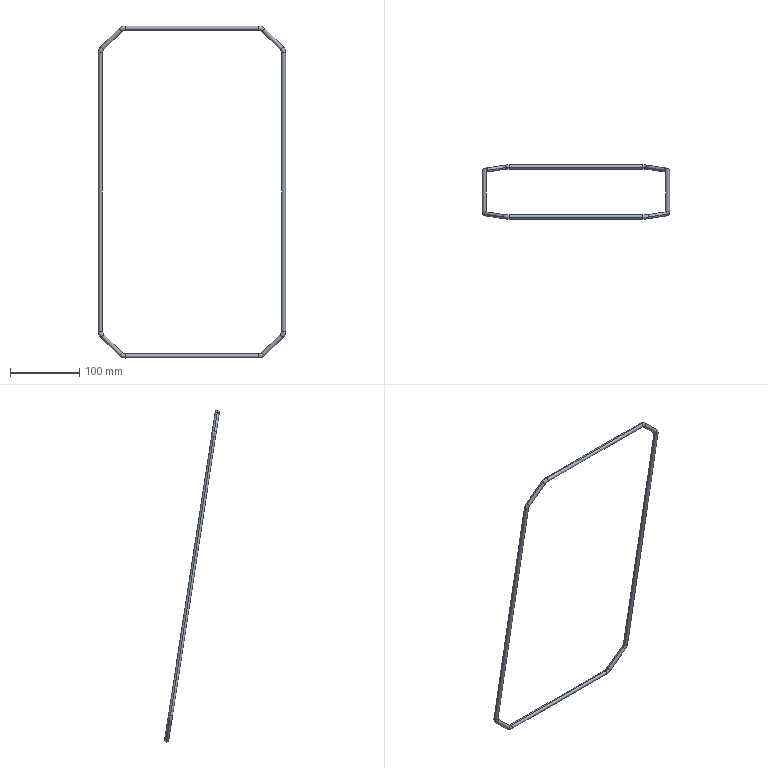Part | SolidWorks | features BaseBody 1 | 1 solid | 32 faces | box 271 x 79.199 x 480.386 mm | volume 39917 mm3 | torus 16 | cylinder 16 | commonest cylinder face diameters 6 x16
STEP:
#1=CARTESIAN_POINT('',(-509.93,505.658,-821.226));
#2=VERTEX_POINT('',#1);
#3=CARTESIAN_POINT('',(-513.445,504.364,-812.84));
#4=VERTEX_POINT('',#3);
#5=CARTESIAN_POINT('',(-501.445,504.364,-812.84));
#6=DIRECTION('',(0.,0.9883,0.1525));
#7=DIRECTION('',(-0.7071,0.1078,-0.6988));
#8=AXIS2_PLACEMENT_3D('',#5,#6,#7);
#9=CIRCLE('',#8,12.);
#10=EDGE_CURVE('',#2,#4,#9,.T.);
#11=ORIENTED_EDGE('',*,*,#10,.T.);
#12=CARTESIAN_POINT('',(-507.445,504.364,-812.84));
#13=VERTEX_POINT('',#12);
#14=CARTESIAN_POINT('',(-510.445,504.364,-812.84));
#15=DIRECTION('',(-0.000000028,-0.1525,0.9883));
#16=DIRECTION('',(1.,-0.000000004,0.000000028));
#17=AXIS2_PLACEMENT_3D('',#14,#15,#16);
#18=CIRCLE('',#17,3.);
#19=EDGE_CURVE('',#13,#4,#18,.T.);
#20=ORIENTED_EDGE('',*,*,#19,.F.);
#21=CARTESIAN_POINT('',(-505.688,505.011,-817.033));
#22=VERTEX_POINT('',#21);
#23=CARTESIAN_POINT('',(-501.445,504.364,-812.84));
#24=DIRECTION('',(0.,0.9883,0.1525));
#25=DIRECTION('',(-0.7071,0.1078,-0.6988));
#26=AXIS2_PLACEMENT_3D('',#23,#24,#25);
#27=CIRCLE('',#26,6.);
#28=EDGE_CURVE('',#22,#13,#27,.T.);
#29=ORIENTED_EDGE('',*,*,#28,.F.);
#30=CARTESIAN_POINT('',(-507.809,505.335,-819.13));
#31=DIRECTION('',(0.7071,0.1078,-0.6988));
#32=DIRECTION('',(-0.7071,0.1078,-0.6988));
#33=AXIS2_PLACEMENT_3D('',#30,#31,#32);
#34=CIRCLE('',#33,3.);
#35=EDGE_CURVE('',#2,#22,#34,.T.);
#36=ORIENTED_EDGE('',*,*,#35,.F.);
#37=EDGE_LOOP('',(#11,#20,#29,#36));
#38=FACE_OUTER_BOUND('',#37,.T.);
#39=CARTESIAN_POINT('',(-501.445,504.364,-812.84));
#40=DIRECTION('',(0.,0.9883,0.1525));
#41=DIRECTION('',(0.7071,-0.1078,0.6988));
#42=AXIS2_PLACEMENT_3D('',#39,#40,#41);
#43=TOROIDAL_SURFACE('',#42,9.,3.);
#44=ADVANCED_FACE('',(#38),#43,.T.);
#45=CARTESIAN_POINT('',(-483.134,509.744,-847.709));
#46=VERTEX_POINT('',#45);
#47=CARTESIAN_POINT('',(-483.134,509.744,-847.709));
#48=DIRECTION('',(-0.7071,-0.1078,0.6988));
#49=VECTOR('',#48,1000.);
#50=LINE('',#47,#49);
#51=EDGE_CURVE('',#46,#2,#50,.T.);
#52=ORIENTED_EDGE('',*,*,#51,.T.);
#53=ORIENTED_EDGE('',*,*,#35,.T.);
#54=CARTESIAN_POINT('',(-478.891,509.097,-843.516));
#55=VERTEX_POINT('',#54);
#56=CARTESIAN_POINT('',(-478.891,509.097,-843.516));
#57=DIRECTION('',(-0.7071,-0.1078,0.6988));
#58=VECTOR('',#57,1000.);
#59=LINE('',#56,#58);
#60=EDGE_CURVE('',#55,#22,#59,.T.);
#61=ORIENTED_EDGE('',*,*,#60,.F.);
#62=CARTESIAN_POINT('',(-481.013,509.421,-845.613));
#63=DIRECTION('',(-0.7071,-0.1078,0.6988));
#64=DIRECTION('',(0.7071,-0.1078,0.6988));
#65=AXIS2_PLACEMENT_3D('',#62,#63,#64);
#66=CIRCLE('',#65,3.);
#67=EDGE_CURVE('',#55,#46,#66,.T.);
#68=ORIENTED_EDGE('',*,*,#67,.T.);
#69=EDGE_LOOP('',(#52,#53,#61,#68));
#70=FACE_OUTER_BOUND('',#69,.T.);
#71=CARTESIAN_POINT('',(-481.013,509.421,-845.613));
#72=DIRECTION('',(-0.7071,-0.1078,0.6988));
#73=DIRECTION('',(-0.7071,0.1078,-0.6988));
#74=AXIS2_PLACEMENT_3D('',#71,#72,#73);
#75=CYLINDRICAL_SURFACE('',#74,3.);
#76=ADVANCED_FACE('',(#70),#75,.T.);
#77=CARTESIAN_POINT('',(-474.649,510.28,-851.183));
#78=VERTEX_POINT('',#77);
#79=CARTESIAN_POINT('',(-474.649,508.45,-839.323));
#80=DIRECTION('',(0.,0.9883,0.1525));
#81=DIRECTION('',(0.,0.1525,-0.9883));
#82=AXIS2_PLACEMENT_3D('',#79,#80,#81);
#83=CIRCLE('',#82,12.);
#84=EDGE_CURVE('',#78,#46,#83,.T.);
#85=ORIENTED_EDGE('',*,*,#84,.T.);
#86=ORIENTED_EDGE('',*,*,#67,.F.);
#87=CARTESIAN_POINT('',(-474.649,509.365,-845.253));
#88=VERTEX_POINT('',#87);
#89=CARTESIAN_POINT('',(-474.649,508.45,-839.323));
#90=DIRECTION('',(0.,0.9883,0.1525));
#91=DIRECTION('',(0.,0.1525,-0.9883));
#92=AXIS2_PLACEMENT_3D('',#89,#90,#91);
#93=CIRCLE('',#92,6.);
#94=EDGE_CURVE('',#88,#55,#93,.T.);
#95=ORIENTED_EDGE('',*,*,#94,.F.);
#96=CARTESIAN_POINT('',(-474.649,509.823,-848.218));
#97=DIRECTION('',(1.,0.,0.));
#98=DIRECTION('',(0.,0.1525,-0.9883));
#99=AXIS2_PLACEMENT_3D('',#96,#97,#98);
#100=CIRCLE('',#99,3.);
#101=EDGE_CURVE('',#78,#88,#100,.T.);
#102=ORIENTED_EDGE('',*,*,#101,.F.);
#103=EDGE_LOOP('',(#85,#86,#95,#102));
#104=FACE_OUTER_BOUND('',#103,.T.);
#105=CARTESIAN_POINT('',(-474.649,508.45,-839.323));
#106=DIRECTION('',(0.,0.9883,0.1525));
#107=DIRECTION('',(0.000000004,-0.1525,0.9883));
#108=AXIS2_PLACEMENT_3D('',#105,#106,#107);
#109=TOROIDAL_SURFACE('',#108,9.,3.);
#110=ADVANCED_FACE('',(#104),#109,.T.);
#111=CARTESIAN_POINT('',(-281.241,510.28,-851.183));
#112=VERTEX_POINT('',#111);
#113=CARTESIAN_POINT('',(-281.241,510.28,-851.183));
#114=DIRECTION('',(-1.,0.,0.));
#115=VECTOR('',#114,1000.);
#116=LINE('',#113,#115);
#117=EDGE_CURVE('',#112,#78,#116,.T.);
#118=ORIENTED_EDGE('',*,*,#117,.T.);
#119=ORIENTED_EDGE('',*,*,#101,.T.);
#120=CARTESIAN_POINT('',(-281.241,509.365,-845.253));
#121=VERTEX_POINT('',#120);
#122=CARTESIAN_POINT('',(-281.241,509.365,-845.253));
#123=DIRECTION('',(-1.,0.,0.));
#124=VECTOR('',#123,1000.);
#125=LINE('',#122,#124);
#126=EDGE_CURVE('',#121,#88,#125,.T.);
#127=ORIENTED_EDGE('',*,*,#126,.F.);
#128=CARTESIAN_POINT('',(-281.241,509.823,-848.218));
#129=DIRECTION('',(-1.,-0.000000001,0.000000004));
#130=DIRECTION('',(0.000000004,-0.1525,0.9883));
#131=AXIS2_PLACEMENT_3D('',#128,#129,#130);
#132=CIRCLE('',#131,3.);
#133=EDGE_CURVE('',#121,#112,#132,.T.);
#134=ORIENTED_EDGE('',*,*,#133,.T.);
#135=EDGE_LOOP('',(#118,#119,#127,#134));
#136=FACE_OUTER_BOUND('',#135,.T.);
#137=CARTESIAN_POINT('',(-281.241,509.823,-848.218));
#138=DIRECTION('',(-1.,0.,0.));
#139=DIRECTION('',(0.,0.1525,-0.9883));
#140=AXIS2_PLACEMENT_3D('',#137,#138,#139);
#141=CYLINDRICAL_SURFACE('',#140,3.);
#142=ADVANCED_FACE('',(#136),#141,.T.);
#143=CARTESIAN_POINT('',(-272.756,509.744,-847.709));
#144=VERTEX_POINT('',#143);
#145=CARTESIAN_POINT('',(-281.241,508.45,-839.323));
#146=DIRECTION('',(0.,0.9883,0.1525));
#147=DIRECTION('',(0.7071,0.1078,-0.6988));
#148=AXIS2_PLACEMENT_3D('',#145,#146,#147);
#149=CIRCLE('',#148,12.);
#150=EDGE_CURVE('',#144,#112,#149,.T.);
#151=ORIENTED_EDGE('',*,*,#150,.T.);
#152=ORIENTED_EDGE('',*,*,#133,.F.);
#153=CARTESIAN_POINT('',(-276.999,509.097,-843.516));
#154=VERTEX_POINT('',#153);
#155=CARTESIAN_POINT('',(-281.241,508.45,-839.323));
#156=DIRECTION('',(0.,0.9883,0.1525));
#157=DIRECTION('',(0.7071,0.1078,-0.6988));
#158=AXIS2_PLACEMENT_3D('',#155,#156,#157);
#159=CIRCLE('',#158,6.);
#160=EDGE_CURVE('',#154,#121,#159,.T.);
#161=ORIENTED_EDGE('',*,*,#160,.F.);
#162=CARTESIAN_POINT('',(-274.878,509.421,-845.613));
#163=DIRECTION('',(0.7071,-0.1078,0.6988));
#164=DIRECTION('',(0.7071,0.1078,-0.6988));
#165=AXIS2_PLACEMENT_3D('',#162,#163,#164);
#166=CIRCLE('',#165,3.);
#167=EDGE_CURVE('',#144,#154,#166,.T.);
#168=ORIENTED_EDGE('',*,*,#167,.F.);
#169=EDGE_LOOP('',(#151,#152,#161,#168));
#170=FACE_OUTER_BOUND('',#169,.T.);
#171=CARTESIAN_POINT('',(-281.241,508.45,-839.323));
#172=DIRECTION('',(0.,0.9883,0.1525));
#173=DIRECTION('',(-0.7071,-0.1078,0.6988));
#174=AXIS2_PLACEMENT_3D('',#171,#172,#173);
#175=TOROIDAL_SURFACE('',#174,9.,3.);
#176=ADVANCED_FACE('',(#170),#175,.T.);
#177=CARTESIAN_POINT('',(-245.96,505.658,-821.226));
#178=VERTEX_POINT('',#177);
#179=CARTESIAN_POINT('',(-245.96,505.658,-821.226));
#180=DIRECTION('',(-0.7071,0.1078,-0.6988));
#181=VECTOR('',#180,1000.);
#182=LINE('',#179,#181);
#183=EDGE_CURVE('',#178,#144,#182,.T.);
#184=ORIENTED_EDGE('',*,*,#183,.T.);
#185=ORIENTED_EDGE('',*,*,#167,.T.);
#186=CARTESIAN_POINT('',(-250.202,505.011,-817.033));
#187=VERTEX_POINT('',#186);
#188=CARTESIAN_POINT('',(-250.202,505.011,-817.033));
#189=DIRECTION('',(-0.7071,0.1078,-0.6988));
#190=VECTOR('',#189,1000.);
#191=LINE('',#188,#190);
#192=EDGE_CURVE('',#187,#154,#191,.T.);
#193=ORIENTED_EDGE('',*,*,#192,.F.);
#194=CARTESIAN_POINT('',(-248.081,505.335,-819.13));
#195=DIRECTION('',(-0.7071,0.1078,-0.6988));
#196=DIRECTION('',(-0.7071,-0.1078,0.6988));
#197=AXIS2_PLACEMENT_3D('',#194,#195,#196);
#198=CIRCLE('',#197,3.);
#199=EDGE_CURVE('',#187,#178,#198,.T.);
#200=ORIENTED_EDGE('',*,*,#199,.T.);
#201=EDGE_LOOP('',(#184,#185,#193,#200));
#202=FACE_OUTER_BOUND('',#201,.T.);
#203=CARTESIAN_POINT('',(-248.081,505.335,-819.13));
#204=DIRECTION('',(-0.7071,0.1078,-0.6988));
#205=DIRECTION('',(0.7071,0.1078,-0.6988));
#206=AXIS2_PLACEMENT_3D('',#203,#204,#205);
#207=CYLINDRICAL_SURFACE('',#206,3.);
#208=ADVANCED_FACE('',(#202),#207,.T.);
#209=CARTESIAN_POINT('',(-242.445,504.364,-812.84));
#210=VERTEX_POINT('',#209);
#211=CARTESIAN_POINT('',(-254.445,504.364,-812.84));
#212=DIRECTION('',(0.,0.9883,0.1525));
#213=DIRECTION('',(1.,0.,0.));
#214=AXIS2_PLACEMENT_3D('',#211,#212,#213);
#215=CIRCLE('',#214,12.);
#216=EDGE_CURVE('',#210,#178,#215,.T.);
#217=ORIENTED_EDGE('',*,*,#216,.T.);
#218=ORIENTED_EDGE('',*,*,#199,.F.);
#219=CARTESIAN_POINT('',(-248.445,504.364,-812.84));
#220=VERTEX_POINT('',#219);
#221=CARTESIAN_POINT('',(-254.445,504.364,-812.84));
#222=DIRECTION('',(0.,0.9883,0.1525));
#223=DIRECTION('',(1.,0.,0.));
#224=AXIS2_PLACEMENT_3D('',#221,#222,#223);
#225=CIRCLE('',#224,6.);
#226=EDGE_CURVE('',#220,#187,#225,.T.);
#227=ORIENTED_EDGE('',*,*,#226,.F.);
#228=CARTESIAN_POINT('',(-245.445,504.364,-812.84));
#229=DIRECTION('',(0.,-0.1525,0.9883));
#230=DIRECTION('',(1.,0.,0.));
#231=AXIS2_PLACEMENT_3D('',#228,#229,#230);
#232=CIRCLE('',#231,3.);
#233=EDGE_CURVE('',#210,#220,#232,.T.);
#234=ORIENTED_EDGE('',*,*,#233,.F.);
#235=EDGE_LOOP('',(#217,#218,#227,#234));
#236=FACE_OUTER_BOUND('',#235,.T.);
#237=CARTESIAN_POINT('',(-254.445,504.364,-812.84));
#238=DIRECTION('',(0.,0.9883,0.1525));
#239=DIRECTION('',(-1.,-0.000000002,0.000000011));
#240=AXIS2_PLACEMENT_3D('',#237,#238,#239);
#241=TOROIDAL_SURFACE('',#240,9.,3.);
#242=ADVANCED_FACE('',(#236),#241,.T.);
#243=CARTESIAN_POINT('',(-242.445,442.083,-409.21));
#244=VERTEX_POINT('',#243);
#245=CARTESIAN_POINT('',(-242.445,442.083,-409.21));
#246=DIRECTION('',(0.,0.1525,-0.9883));
#247=VECTOR('',#246,1000.);
#248=LINE('',#245,#247);
#249=EDGE_CURVE('',#244,#210,#248,.T.);
#250=ORIENTED_EDGE('',*,*,#249,.T.);
#251=ORIENTED_EDGE('',*,*,#233,.T.);
#252=CARTESIAN_POINT('',(-248.445,442.083,-409.21));
#253=VERTEX_POINT('',#252);
#254=CARTESIAN_POINT('',(-248.445,442.083,-409.21));
#255=DIRECTION('',(0.,0.1525,-0.9883));
#256=VECTOR('',#255,1000.);
#257=LINE('',#254,#256);
#258=EDGE_CURVE('',#253,#220,#257,.T.);
#259=ORIENTED_EDGE('',*,*,#258,.F.);
#260=CARTESIAN_POINT('',(-245.445,442.083,-409.21));
#261=DIRECTION('',(-0.000000004,0.1525,-0.9883));
#262=DIRECTION('',(-1.,-0.000000001,0.000000004));
#263=AXIS2_PLACEMENT_3D('',#260,#261,#262);
#264=CIRCLE('',#263,3.);
#265=EDGE_CURVE('',#253,#244,#264,.T.);
#266=ORIENTED_EDGE('',*,*,#265,.T.);
#267=EDGE_LOOP('',(#250,#251,#259,#266));
#268=FACE_OUTER_BOUND('',#267,.T.);
#269=CARTESIAN_POINT('',(-245.445,442.083,-409.21));
#270=DIRECTION('',(0.,0.1525,-0.9883));
#271=DIRECTION('',(1.,0.,0.));
#272=AXIS2_PLACEMENT_3D('',#269,#270,#271);
#273=CYLINDRICAL_SURFACE('',#272,3.);
#274=ADVANCED_FACE('',(#268),#273,.T.);
#275=CARTESIAN_POINT('',(-245.96,440.789,-400.823));
#276=VERTEX_POINT('',#275);
#277=CARTESIAN_POINT('',(-254.445,442.083,-409.21));
#278=DIRECTION('',(0.,0.9883,0.1525));
#279=DIRECTION('',(0.7071,-0.1078,0.6988));
#280=AXIS2_PLACEMENT_3D('',#277,#278,#279);
#281=CIRCLE('',#280,12.);
#282=EDGE_CURVE('',#276,#244,#281,.T.);
#283=ORIENTED_EDGE('',*,*,#282,.T.);
#284=ORIENTED_EDGE('',*,*,#265,.F.);
#285=CARTESIAN_POINT('',(-250.202,441.436,-405.017));
#286=VERTEX_POINT('',#285);
#287=CARTESIAN_POINT('',(-254.445,442.083,-409.21));
#288=DIRECTION('',(0.,0.9883,0.1525));
#289=DIRECTION('',(0.7071,-0.1078,0.6988));
#290=AXIS2_PLACEMENT_3D('',#287,#288,#289);
#291=CIRCLE('',#290,6.);
#292=EDGE_CURVE('',#286,#253,#291,.T.);
#293=ORIENTED_EDGE('',*,*,#292,.F.);
#294=CARTESIAN_POINT('',(-248.081,441.113,-402.92));
#295=DIRECTION('',(-0.7071,-0.1078,0.6988));
#296=DIRECTION('',(0.7071,-0.1078,0.6988));
#297=AXIS2_PLACEMENT_3D('',#294,#295,#296);
#298=CIRCLE('',#297,3.);
#299=EDGE_CURVE('',#276,#286,#298,.T.);
#300=ORIENTED_EDGE('',*,*,#299,.F.);
#301=EDGE_LOOP('',(#283,#284,#293,#300));
#302=FACE_OUTER_BOUND('',#301,.T.);
#303=CARTESIAN_POINT('',(-254.445,442.083,-409.21));
#304=DIRECTION('',(0.,0.9883,0.1525));
#305=DIRECTION('',(-0.7071,0.1078,-0.6988));
#306=AXIS2_PLACEMENT_3D('',#303,#304,#305);
#307=TOROIDAL_SURFACE('',#306,9.,3.);
#308=ADVANCED_FACE('',(#302),#307,.T.);
#309=CARTESIAN_POINT('',(-272.756,436.703,-374.341));
#310=VERTEX_POINT('',#309);
#311=CARTESIAN_POINT('',(-272.756,436.703,-374.341));
#312=DIRECTION('',(0.7071,0.1078,-0.6988));
#313=VECTOR('',#312,1000.);
#314=LINE('',#311,#313);
#315=EDGE_CURVE('',#310,#276,#314,.T.);
#316=ORIENTED_EDGE('',*,*,#315,.T.);
#317=ORIENTED_EDGE('',*,*,#299,.T.);
#318=CARTESIAN_POINT('',(-276.999,437.35,-378.534));
#319=VERTEX_POINT('',#318);
#320=CARTESIAN_POINT('',(-276.999,437.35,-378.534));
#321=DIRECTION('',(0.7071,0.1078,-0.6988));
#322=VECTOR('',#321,1000.);
#323=LINE('',#320,#322);
#324=EDGE_CURVE('',#319,#286,#323,.T.);
#325=ORIENTED_EDGE('',*,*,#324,.F.);
#326=CARTESIAN_POINT('',(-274.878,437.026,-376.437));
#327=DIRECTION('',(0.7071,0.1078,-0.6988));
#328=DIRECTION('',(-0.7071,0.1078,-0.6988));
#329=AXIS2_PLACEMENT_3D('',#326,#327,#328);
#330=CIRCLE('',#329,3.);
#331=EDGE_CURVE('',#319,#310,#330,.T.);
#332=ORIENTED_EDGE('',*,*,#331,.T.);
#333=EDGE_LOOP('',(#316,#317,#325,#332));
#334=FACE_OUTER_BOUND('',#333,.T.);
#335=CARTESIAN_POINT('',(-274.878,437.026,-376.437));
#336=DIRECTION('',(0.7071,0.1078,-0.6988));
#337=DIRECTION('',(0.7071,-0.1078,0.6988));
#338=AXIS2_PLACEMENT_3D('',#335,#336,#337);
#339=CYLINDRICAL_SURFACE('',#338,3.);
#340=ADVANCED_FACE('',(#334),#339,.T.);
#341=CARTESIAN_POINT('',(-281.241,436.167,-370.867));
#342=VERTEX_POINT('',#341);
#343=CARTESIAN_POINT('',(-281.241,437.997,-382.727));
#344=DIRECTION('',(0.,0.9883,0.1525));
#345=DIRECTION('',(0.,-0.1525,0.9883));
#346=AXIS2_PLACEMENT_3D('',#343,#344,#345);
#347=CIRCLE('',#346,12.);
#348=EDGE_CURVE('',#342,#310,#347,.T.);
#349=ORIENTED_EDGE('',*,*,#348,.T.);
#350=ORIENTED_EDGE('',*,*,#331,.F.);
#351=CARTESIAN_POINT('',(-281.241,437.082,-376.797));
#352=VERTEX_POINT('',#351);
#353=CARTESIAN_POINT('',(-281.241,437.997,-382.727));
#354=DIRECTION('',(0.,0.9883,0.1525));
#355=DIRECTION('',(0.,-0.1525,0.9883));
#356=AXIS2_PLACEMENT_3D('',#353,#354,#355);
#357=CIRCLE('',#356,6.);
#358=EDGE_CURVE('',#352,#319,#357,.T.);
#359=ORIENTED_EDGE('',*,*,#358,.F.);
#360=CARTESIAN_POINT('',(-281.241,436.624,-373.832));
#361=DIRECTION('',(-1.,0.,0.));
#362=DIRECTION('',(0.,-0.1525,0.9883));
#363=AXIS2_PLACEMENT_3D('',#360,#361,#362);
#364=CIRCLE('',#363,3.);
#365=EDGE_CURVE('',#342,#352,#364,.T.);
#366=ORIENTED_EDGE('',*,*,#365,.F.);
#367=EDGE_LOOP('',(#349,#350,#359,#366));
#368=FACE_OUTER_BOUND('',#367,.T.);
#369=CARTESIAN_POINT('',(-281.241,437.997,-382.727));
#370=DIRECTION('',(0.,0.9883,0.1525));
#371=DIRECTION('',(-0.000000004,0.1525,-0.9883));
#372=AXIS2_PLACEMENT_3D('',#369,#370,#371);
#373=TOROIDAL_SURFACE('',#372,9.,3.);
#374=ADVANCED_FACE('',(#368),#373,.T.);
#375=CARTESIAN_POINT('',(-474.649,436.167,-370.867));
#376=VERTEX_POINT('',#375);
#377=CARTESIAN_POINT('',(-474.649,436.167,-370.867));
#378=DIRECTION('',(1.,0.,0.));
#379=VECTOR('',#378,1000.);
#380=LINE('',#377,#379);
#381=EDGE_CURVE('',#376,#342,#380,.T.);
#382=ORIENTED_EDGE('',*,*,#381,.T.);
#383=ORIENTED_EDGE('',*,*,#365,.T.);
#384=CARTESIAN_POINT('',(-474.649,437.082,-376.797));
#385=VERTEX_POINT('',#384);
#386=CARTESIAN_POINT('',(-474.649,437.082,-376.797));
#387=DIRECTION('',(1.,0.,0.));
#388=VECTOR('',#387,1000.);
#389=LINE('',#386,#388);
#390=EDGE_CURVE('',#385,#352,#389,.T.);
#391=ORIENTED_EDGE('',*,*,#390,.F.);
#392=CARTESIAN_POINT('',(-474.649,436.624,-373.832));
#393=DIRECTION('',(1.,-0.000000002,0.000000012));
#394=DIRECTION('',(0.000000012,0.1525,-0.9883));
#395=AXIS2_PLACEMENT_3D('',#392,#393,#394);
#396=CIRCLE('',#395,3.);
#397=EDGE_CURVE('',#385,#376,#396,.T.);
#398=ORIENTED_EDGE('',*,*,#397,.T.);
#399=EDGE_LOOP('',(#382,#383,#391,#398));
#400=FACE_OUTER_BOUND('',#399,.T.);
#401=CARTESIAN_POINT('',(-474.649,436.624,-373.832));
#402=DIRECTION('',(1.,0.,0.));
#403=DIRECTION('',(0.,-0.1525,0.9883));
#404=AXIS2_PLACEMENT_3D('',#401,#402,#403);
#405=CYLINDRICAL_SURFACE('',#404,3.);
#406=ADVANCED_FACE('',(#400),#405,.T.);
#407=CARTESIAN_POINT('',(-483.134,436.703,-374.341));
#408=VERTEX_POINT('',#407);
#409=CARTESIAN_POINT('',(-474.649,437.997,-382.727));
#410=DIRECTION('',(0.,0.9883,0.1525));
#411=DIRECTION('',(-0.7071,-0.1078,0.6988));
#412=AXIS2_PLACEMENT_3D('',#409,#410,#411);
#413=CIRCLE('',#412,12.);
#414=EDGE_CURVE('',#408,#376,#413,.T.);
#415=ORIENTED_EDGE('',*,*,#414,.T.);
#416=ORIENTED_EDGE('',*,*,#397,.F.);
#417=CARTESIAN_POINT('',(-478.891,437.35,-378.534));
#418=VERTEX_POINT('',#417);
#419=CARTESIAN_POINT('',(-474.649,437.997,-382.727));
#420=DIRECTION('',(0.,0.9883,0.1525));
#421=DIRECTION('',(-0.7071,-0.1078,0.6988));
#422=AXIS2_PLACEMENT_3D('',#419,#420,#421);
#423=CIRCLE('',#422,6.);
#424=EDGE_CURVE('',#418,#385,#423,.T.);
#425=ORIENTED_EDGE('',*,*,#424,.F.);
#426=CARTESIAN_POINT('',(-481.013,437.026,-376.437));
#427=DIRECTION('',(-0.7071,0.1078,-0.6988));
#428=DIRECTION('',(-0.7071,-0.1078,0.6988));
#429=AXIS2_PLACEMENT_3D('',#426,#427,#428);
#430=CIRCLE('',#429,3.);
#431=EDGE_CURVE('',#408,#418,#430,.T.);
#432=ORIENTED_EDGE('',*,*,#431,.F.);
#433=EDGE_LOOP('',(#415,#416,#425,#432));
#434=FACE_OUTER_BOUND('',#433,.T.);
#435=CARTESIAN_POINT('',(-474.649,437.997,-382.727));
#436=DIRECTION('',(0.,0.9883,0.1525));
#437=DIRECTION('',(0.7071,0.1078,-0.6988));
#438=AXIS2_PLACEMENT_3D('',#435,#436,#437);
#439=TOROIDAL_SURFACE('',#438,9.,3.);
#440=ADVANCED_FACE('',(#434),#439,.T.);
#441=CARTESIAN_POINT('',(-509.93,440.789,-400.823));
#442=VERTEX_POINT('',#441);
#443=CARTESIAN_POINT('',(-509.93,440.789,-400.823));
#444=DIRECTION('',(0.7071,-0.1078,0.6988));
#445=VECTOR('',#444,1000.);
#446=LINE('',#443,#445);
#447=EDGE_CURVE('',#442,#408,#446,.T.);
#448=ORIENTED_EDGE('',*,*,#447,.T.);
#449=ORIENTED_EDGE('',*,*,#431,.T.);
#450=CARTESIAN_POINT('',(-505.688,441.436,-405.017));
#451=VERTEX_POINT('',#450);
#452=CARTESIAN_POINT('',(-505.688,441.436,-405.017));
#453=DIRECTION('',(0.7071,-0.1078,0.6988));
#454=VECTOR('',#453,1000.);
#455=LINE('',#452,#454);
#456=EDGE_CURVE('',#451,#418,#455,.T.);
#457=ORIENTED_EDGE('',*,*,#456,.F.);
#458=CARTESIAN_POINT('',(-507.809,441.113,-402.92));
#459=DIRECTION('',(0.7071,-0.1078,0.6988));
#460=DIRECTION('',(0.7071,0.1078,-0.6988));
#461=AXIS2_PLACEMENT_3D('',#458,#459,#460);
#462=CIRCLE('',#461,3.);
#463=EDGE_CURVE('',#451,#442,#462,.T.);
#464=ORIENTED_EDGE('',*,*,#463,.T.);
#465=EDGE_LOOP('',(#448,#449,#457,#464));
#466=FACE_OUTER_BOUND('',#465,.T.);
#467=CARTESIAN_POINT('',(-507.809,441.113,-402.92));
#468=DIRECTION('',(0.7071,-0.1078,0.6988));
#469=DIRECTION('',(-0.7071,-0.1078,0.6988));
#470=AXIS2_PLACEMENT_3D('',#467,#468,#469);
#471=CYLINDRICAL_SURFACE('',#470,3.);
#472=ADVANCED_FACE('',(#466),#471,.T.);
#473=CARTESIAN_POINT('',(-513.445,442.083,-409.21));
#474=VERTEX_POINT('',#473);
#475=CARTESIAN_POINT('',(-501.445,442.083,-409.21));
#476=DIRECTION('',(0.,0.9883,0.1525));
#477=DIRECTION('',(-1.,0.,0.));
#478=AXIS2_PLACEMENT_3D('',#475,#476,#477);
#479=CIRCLE('',#478,12.);
#480=EDGE_CURVE('',#474,#442,#479,.T.);
#481=ORIENTED_EDGE('',*,*,#480,.T.);
#482=ORIENTED_EDGE('',*,*,#463,.F.);
#483=CARTESIAN_POINT('',(-507.445,442.083,-409.21));
#484=VERTEX_POINT('',#483);
#485=CARTESIAN_POINT('',(-501.445,442.083,-409.21));
#486=DIRECTION('',(0.,0.9883,0.1525));
#487=DIRECTION('',(-1.,0.,0.));
#488=AXIS2_PLACEMENT_3D('',#485,#486,#487);
#489=CIRCLE('',#488,6.);
#490=EDGE_CURVE('',#484,#451,#489,.T.);
#491=ORIENTED_EDGE('',*,*,#490,.F.);
#492=CARTESIAN_POINT('',(-510.445,442.083,-409.21));
#493=DIRECTION('',(0.,0.1525,-0.9883));
#494=DIRECTION('',(-1.,0.,0.));
#495=AXIS2_PLACEMENT_3D('',#492,#493,#494);
#496=CIRCLE('',#495,3.);
#497=EDGE_CURVE('',#474,#484,#496,.T.);
#498=ORIENTED_EDGE('',*,*,#497,.F.);
#499=EDGE_LOOP('',(#481,#482,#491,#498));
#500=FACE_OUTER_BOUND('',#499,.T.);
#501=CARTESIAN_POINT('',(-501.445,442.083,-409.21));
#502=DIRECTION('',(0.,0.9883,0.1525));
#503=DIRECTION('',(1.,0.000000002,-0.000000011));
#504=AXIS2_PLACEMENT_3D('',#501,#502,#503);
#505=TOROIDAL_SURFACE('',#504,9.,3.);
#506=ADVANCED_FACE('',(#500),#505,.T.);
#507=CARTESIAN_POINT('',(-513.445,504.364,-812.84));
#508=DIRECTION('',(0.,-0.1525,0.9883));
#509=VECTOR('',#508,1000.);
#510=LINE('',#507,#509);
#511=EDGE_CURVE('',#4,#474,#510,.T.);
#512=ORIENTED_EDGE('',*,*,#511,.T.);
#513=ORIENTED_EDGE('',*,*,#497,.T.);
#514=CARTESIAN_POINT('',(-507.445,504.364,-812.84));
#515=DIRECTION('',(0.,-0.1525,0.9883));
#516=VECTOR('',#515,1000.);
#517=LINE('',#514,#516);
#518=EDGE_CURVE('',#13,#484,#517,.T.);
#519=ORIENTED_EDGE('',*,*,#518,.F.);
#520=ORIENTED_EDGE('',*,*,#19,.T.);
#521=EDGE_LOOP('',(#512,#513,#519,#520));
#522=FACE_OUTER_BOUND('',#521,.T.);
#523=CARTESIAN_POINT('',(-510.445,504.364,-812.84));
#524=DIRECTION('',(0.,-0.1525,0.9883));
#525=DIRECTION('',(-1.,0.,0.));
#526=AXIS2_PLACEMENT_3D('',#523,#524,#525);
#527=CYLINDRICAL_SURFACE('',#526,3.);
#528=ADVANCED_FACE('',(#522),#527,.T.);
#529=ORIENTED_EDGE('',*,*,#518,.T.);
#530=CARTESIAN_POINT('',(-510.445,442.083,-409.21));
#531=DIRECTION('',(0.,0.1525,-0.9883));
#532=DIRECTION('',(1.,0.,0.));
#533=AXIS2_PLACEMENT_3D('',#530,#531,#532);
#534=CIRCLE('',#533,3.);
#535=EDGE_CURVE('',#484,#474,#534,.T.);
#536=ORIENTED_EDGE('',*,*,#535,.T.);
#537=ORIENTED_EDGE('',*,*,#511,.F.);
#538=CARTESIAN_POINT('',(-510.445,504.364,-812.84));
#539=DIRECTION('',(-0.000000028,-0.1525,0.9883));
#540=DIRECTION('',(-1.,0.000000004,-0.000000028));
#541=AXIS2_PLACEMENT_3D('',#538,#539,#540);
#542=CIRCLE('',#541,3.);
#543=EDGE_CURVE('',#4,#13,#542,.T.);
#544=ORIENTED_EDGE('',*,*,#543,.T.);
#545=EDGE_LOOP('',(#529,#536,#537,#544));
#546=FACE_OUTER_BOUND('',#545,.T.);
#547=CARTESIAN_POINT('',(-510.445,504.364,-812.84));
#548=DIRECTION('',(0.,-0.1525,0.9883));
#549=DIRECTION('',(-1.,0.,0.));
#550=AXIS2_PLACEMENT_3D('',#547,#548,#549);
#551=CYLINDRICAL_SURFACE('',#550,3.);
#552=ADVANCED_FACE('',(#546),#551,.T.);
#553=ORIENTED_EDGE('',*,*,#28,.T.);
#554=ORIENTED_EDGE('',*,*,#543,.F.);
#555=ORIENTED_EDGE('',*,*,#10,.F.);
#556=CARTESIAN_POINT('',(-507.809,505.335,-819.13));
#557=DIRECTION('',(0.7071,0.1078,-0.6988));
#558=DIRECTION('',(0.7071,-0.1078,0.6988));
#559=AXIS2_PLACEMENT_3D('',#556,#557,#558);
#560=CIRCLE('',#559,3.);
#561=EDGE_CURVE('',#22,#2,#560,.T.);
#562=ORIENTED_EDGE('',*,*,#561,.F.);
#563=EDGE_LOOP('',(#553,#554,#555,#562));
#564=FACE_OUTER_BOUND('',#563,.T.);
#565=CARTESIAN_POINT('',(-501.445,504.364,-812.84));
#566=DIRECTION('',(0.,0.9883,0.1525));
#567=DIRECTION('',(0.7071,-0.1078,0.6988));
#568=AXIS2_PLACEMENT_3D('',#565,#566,#567);
#569=TOROIDAL_SURFACE('',#568,9.,3.);
#570=ADVANCED_FACE('',(#564),#569,.T.);
#571=ORIENTED_EDGE('',*,*,#60,.T.);
#572=ORIENTED_EDGE('',*,*,#561,.T.);
#573=ORIENTED_EDGE('',*,*,#51,.F.);
#574=CARTESIAN_POINT('',(-481.013,509.421,-845.613));
#575=DIRECTION('',(-0.7071,-0.1078,0.6988));
#576=DIRECTION('',(-0.7071,0.1078,-0.6988));
#577=AXIS2_PLACEMENT_3D('',#574,#575,#576);
#578=CIRCLE('',#577,3.);
#579=EDGE_CURVE('',#46,#55,#578,.T.);
#580=ORIENTED_EDGE('',*,*,#579,.T.);
#581=EDGE_LOOP('',(#571,#572,#573,#580));
#582=FACE_OUTER_BOUND('',#581,.T.);
#583=CARTESIAN_POINT('',(-481.013,509.421,-845.613));
#584=DIRECTION('',(-0.7071,-0.1078,0.6988));
#585=DIRECTION('',(-0.7071,0.1078,-0.6988));
#586=AXIS2_PLACEMENT_3D('',#583,#584,#585);
#587=CYLINDRICAL_SURFACE('',#586,3.);
#588=ADVANCED_FACE('',(#582),#587,.T.);
#589=ORIENTED_EDGE('',*,*,#94,.T.);
#590=ORIENTED_EDGE('',*,*,#579,.F.);
#591=ORIENTED_EDGE('',*,*,#84,.F.);
#592=CARTESIAN_POINT('',(-474.649,509.823,-848.218));
#593=DIRECTION('',(1.,0.,0.));
#594=DIRECTION('',(0.,-0.1525,0.9883));
#595=AXIS2_PLACEMENT_3D('',#592,#593,#594);
#596=CIRCLE('',#595,3.);
#597=EDGE_CURVE('',#88,#78,#596,.T.);
#598=ORIENTED_EDGE('',*,*,#597,.F.);
#599=EDGE_LOOP('',(#589,#590,#591,#598));
#600=FACE_OUTER_BOUND('',#599,.T.);
#601=CARTESIAN_POINT('',(-474.649,508.45,-839.323));
#602=DIRECTION('',(0.,0.9883,0.1525));
#603=DIRECTION('',(0.000000004,-0.1525,0.9883));
#604=AXIS2_PLACEMENT_3D('',#601,#602,#603);
#605=TOROIDAL_SURFACE('',#604,9.,3.);
#606=ADVANCED_FACE('',(#600),#605,.T.);
#607=ORIENTED_EDGE('',*,*,#126,.T.);
#608=ORIENTED_EDGE('',*,*,#597,.T.);
#609=ORIENTED_EDGE('',*,*,#117,.F.);
#610=CARTESIAN_POINT('',(-281.241,509.823,-848.218));
#611=DIRECTION('',(-1.,-0.000000001,0.000000004));
#612=DIRECTION('',(-0.000000004,0.1525,-0.9883));
#613=AXIS2_PLACEMENT_3D('',#610,#611,#612);
#614=CIRCLE('',#613,3.);
#615=EDGE_CURVE('',#112,#121,#614,.T.);
#616=ORIENTED_EDGE('',*,*,#615,.T.);
#617=EDGE_LOOP('',(#607,#608,#609,#616));
#618=FACE_OUTER_BOUND('',#617,.T.);
#619=CARTESIAN_POINT('',(-281.241,509.823,-848.218));
#620=DIRECTION('',(-1.,0.,0.));
#621=DIRECTION('',(0.,0.1525,-0.9883));
#622=AXIS2_PLACEMENT_3D('',#619,#620,#621);
#623=CYLINDRICAL_SURFACE('',#622,3.);
#624=ADVANCED_FACE('',(#618),#623,.T.);
#625=ORIENTED_EDGE('',*,*,#160,.T.);
#626=ORIENTED_EDGE('',*,*,#615,.F.);
#627=ORIENTED_EDGE('',*,*,#150,.F.);
#628=CARTESIAN_POINT('',(-274.878,509.421,-845.613));
#629=DIRECTION('',(0.7071,-0.1078,0.6988));
#630=DIRECTION('',(-0.7071,-0.1078,0.6988));
#631=AXIS2_PLACEMENT_3D('',#628,#629,#630);
#632=CIRCLE('',#631,3.);
#633=EDGE_CURVE('',#154,#144,#632,.T.);
#634=ORIENTED_EDGE('',*,*,#633,.F.);
#635=EDGE_LOOP('',(#625,#626,#627,#634));
#636=FACE_OUTER_BOUND('',#635,.T.);
#637=CARTESIAN_POINT('',(-281.241,508.45,-839.323));
#638=DIRECTION('',(0.,0.9883,0.1525));
#639=DIRECTION('',(-0.7071,-0.1078,0.6988));
#640=AXIS2_PLACEMENT_3D('',#637,#638,#639);
#641=TOROIDAL_SURFACE('',#640,9.,3.);
#642=ADVANCED_FACE('',(#636),#641,.T.);
#643=ORIENTED_EDGE('',*,*,#192,.T.);
#644=ORIENTED_EDGE('',*,*,#633,.T.);
#645=ORIENTED_EDGE('',*,*,#183,.F.);
#646=CARTESIAN_POINT('',(-248.081,505.335,-819.13));
#647=DIRECTION('',(-0.7071,0.1078,-0.6988));
#648=DIRECTION('',(0.7071,0.1078,-0.6988));
#649=AXIS2_PLACEMENT_3D('',#646,#647,#648);
#650=CIRCLE('',#649,3.);
#651=EDGE_CURVE('',#178,#187,#650,.T.);
#652=ORIENTED_EDGE('',*,*,#651,.T.);
#653=EDGE_LOOP('',(#643,#644,#645,#652));
#654=FACE_OUTER_BOUND('',#653,.T.);
#655=CARTESIAN_POINT('',(-248.081,505.335,-819.13));
#656=DIRECTION('',(-0.7071,0.1078,-0.6988));
#657=DIRECTION('',(0.7071,0.1078,-0.6988));
#658=AXIS2_PLACEMENT_3D('',#655,#656,#657);
#659=CYLINDRICAL_SURFACE('',#658,3.);
#660=ADVANCED_FACE('',(#654),#659,.T.);
#661=ORIENTED_EDGE('',*,*,#226,.T.);
#662=ORIENTED_EDGE('',*,*,#651,.F.);
#663=ORIENTED_EDGE('',*,*,#216,.F.);
#664=CARTESIAN_POINT('',(-245.445,504.364,-812.84));
#665=DIRECTION('',(0.,-0.1525,0.9883));
#666=DIRECTION('',(-1.,0.,0.));
#667=AXIS2_PLACEMENT_3D('',#664,#665,#666);
#668=CIRCLE('',#667,3.);
#669=EDGE_CURVE('',#220,#210,#668,.T.);
#670=ORIENTED_EDGE('',*,*,#669,.F.);
#671=EDGE_LOOP('',(#661,#662,#663,#670));
#672=FACE_OUTER_BOUND('',#671,.T.);
#673=CARTESIAN_POINT('',(-254.445,504.364,-812.84));
#674=DIRECTION('',(0.,0.9883,0.1525));
#675=DIRECTION('',(-1.,-0.000000002,0.000000011));
#676=AXIS2_PLACEMENT_3D('',#673,#674,#675);
#677=TOROIDAL_SURFACE('',#676,9.,3.);
#678=ADVANCED_FACE('',(#672),#677,.T.);
#679=ORIENTED_EDGE('',*,*,#258,.T.);
#680=ORIENTED_EDGE('',*,*,#669,.T.);
#681=ORIENTED_EDGE('',*,*,#249,.F.);
#682=CARTESIAN_POINT('',(-245.445,442.083,-409.21));
#683=DIRECTION('',(-0.000000004,0.1525,-0.9883));
#684=DIRECTION('',(1.,0.000000001,-0.000000004));
#685=AXIS2_PLACEMENT_3D('',#682,#683,#684);
#686=CIRCLE('',#685,3.);
#687=EDGE_CURVE('',#244,#253,#686,.T.);
#688=ORIENTED_EDGE('',*,*,#687,.T.);
#689=EDGE_LOOP('',(#679,#680,#681,#688));
#690=FACE_OUTER_BOUND('',#689,.T.);
#691=CARTESIAN_POINT('',(-245.445,442.083,-409.21));
#692=DIRECTION('',(0.,0.1525,-0.9883));
#693=DIRECTION('',(1.,0.,0.));
#694=AXIS2_PLACEMENT_3D('',#691,#692,#693);
#695=CYLINDRICAL_SURFACE('',#694,3.);
#696=ADVANCED_FACE('',(#690),#695,.T.);
#697=ORIENTED_EDGE('',*,*,#292,.T.);
#698=ORIENTED_EDGE('',*,*,#687,.F.);
#699=ORIENTED_EDGE('',*,*,#282,.F.);
#700=CARTESIAN_POINT('',(-248.081,441.113,-402.92));
#701=DIRECTION('',(-0.7071,-0.1078,0.6988));
#702=DIRECTION('',(-0.7071,0.1078,-0.6988));
#703=AXIS2_PLACEMENT_3D('',#700,#701,#702);
#704=CIRCLE('',#703,3.);
#705=EDGE_CURVE('',#286,#276,#704,.T.);
#706=ORIENTED_EDGE('',*,*,#705,.F.);
#707=EDGE_LOOP('',(#697,#698,#699,#706));
#708=FACE_OUTER_BOUND('',#707,.T.);
#709=CARTESIAN_POINT('',(-254.445,442.083,-409.21));
#710=DIRECTION('',(0.,0.9883,0.1525));
#711=DIRECTION('',(-0.7071,0.1078,-0.6988));
#712=AXIS2_PLACEMENT_3D('',#709,#710,#711);
#713=TOROIDAL_SURFACE('',#712,9.,3.);
#714=ADVANCED_FACE('',(#708),#713,.T.);
#715=ORIENTED_EDGE('',*,*,#324,.T.);
#716=ORIENTED_EDGE('',*,*,#705,.T.);
#717=ORIENTED_EDGE('',*,*,#315,.F.);
#718=CARTESIAN_POINT('',(-274.878,437.026,-376.437));
#719=DIRECTION('',(0.7071,0.1078,-0.6988));
#720=DIRECTION('',(0.7071,-0.1078,0.6988));
#721=AXIS2_PLACEMENT_3D('',#718,#719,#720);
#722=CIRCLE('',#721,3.);
#723=EDGE_CURVE('',#310,#319,#722,.T.);
#724=ORIENTED_EDGE('',*,*,#723,.T.);
#725=EDGE_LOOP('',(#715,#716,#717,#724));
#726=FACE_OUTER_BOUND('',#725,.T.);
#727=CARTESIAN_POINT('',(-274.878,437.026,-376.437));
#728=DIRECTION('',(0.7071,0.1078,-0.6988));
#729=DIRECTION('',(0.7071,-0.1078,0.6988));
#730=AXIS2_PLACEMENT_3D('',#727,#728,#729);
#731=CYLINDRICAL_SURFACE('',#730,3.);
#732=ADVANCED_FACE('',(#726),#731,.T.);
#733=ORIENTED_EDGE('',*,*,#358,.T.);
#734=ORIENTED_EDGE('',*,*,#723,.F.);
#735=ORIENTED_EDGE('',*,*,#348,.F.);
#736=CARTESIAN_POINT('',(-281.241,436.624,-373.832));
#737=DIRECTION('',(-1.,0.,0.));
#738=DIRECTION('',(0.,0.1525,-0.9883));
#739=AXIS2_PLACEMENT_3D('',#736,#737,#738);
#740=CIRCLE('',#739,3.);
#741=EDGE_CURVE('',#352,#342,#740,.T.);
#742=ORIENTED_EDGE('',*,*,#741,.F.);
#743=EDGE_LOOP('',(#733,#734,#735,#742));
#744=FACE_OUTER_BOUND('',#743,.T.);
#745=CARTESIAN_POINT('',(-281.241,437.997,-382.727));
#746=DIRECTION('',(0.,0.9883,0.1525));
#747=DIRECTION('',(-0.000000004,0.1525,-0.9883));
#748=AXIS2_PLACEMENT_3D('',#745,#746,#747);
#749=TOROIDAL_SURFACE('',#748,9.,3.);
#750=ADVANCED_FACE('',(#744),#749,.T.);
#751=ORIENTED_EDGE('',*,*,#390,.T.);
#752=ORIENTED_EDGE('',*,*,#741,.T.);
#753=ORIENTED_EDGE('',*,*,#381,.F.);
#754=CARTESIAN_POINT('',(-474.649,436.624,-373.832));
#755=DIRECTION('',(1.,-0.000000002,0.000000012));
#756=DIRECTION('',(-0.000000012,-0.1525,0.9883));
#757=AXIS2_PLACEMENT_3D('',#754,#755,#756);
#758=CIRCLE('',#757,3.);
#759=EDGE_CURVE('',#376,#385,#758,.T.);
#760=ORIENTED_EDGE('',*,*,#759,.T.);
#761=EDGE_LOOP('',(#751,#752,#753,#760));
#762=FACE_OUTER_BOUND('',#761,.T.);
#763=CARTESIAN_POINT('',(-474.649,436.624,-373.832));
#764=DIRECTION('',(1.,0.,0.));
#765=DIRECTION('',(0.,-0.1525,0.9883));
#766=AXIS2_PLACEMENT_3D('',#763,#764,#765);
#767=CYLINDRICAL_SURFACE('',#766,3.);
#768=ADVANCED_FACE('',(#762),#767,.T.);
#769=ORIENTED_EDGE('',*,*,#424,.T.);
#770=ORIENTED_EDGE('',*,*,#759,.F.);
#771=ORIENTED_EDGE('',*,*,#414,.F.);
#772=CARTESIAN_POINT('',(-481.013,437.026,-376.437));
#773=DIRECTION('',(-0.7071,0.1078,-0.6988));
#774=DIRECTION('',(0.7071,0.1078,-0.6988));
#775=AXIS2_PLACEMENT_3D('',#772,#773,#774);
#776=CIRCLE('',#775,3.);
#777=EDGE_CURVE('',#418,#408,#776,.T.);
#778=ORIENTED_EDGE('',*,*,#777,.F.);
#779=EDGE_LOOP('',(#769,#770,#771,#778));
#780=FACE_OUTER_BOUND('',#779,.T.);
#781=CARTESIAN_POINT('',(-474.649,437.997,-382.727));
#782=DIRECTION('',(0.,0.9883,0.1525));
#783=DIRECTION('',(0.7071,0.1078,-0.6988));
#784=AXIS2_PLACEMENT_3D('',#781,#782,#783);
#785=TOROIDAL_SURFACE('',#784,9.,3.);
#786=ADVANCED_FACE('',(#780),#785,.T.);
#787=ORIENTED_EDGE('',*,*,#456,.T.);
#788=ORIENTED_EDGE('',*,*,#777,.T.);
#789=ORIENTED_EDGE('',*,*,#447,.F.);
#790=CARTESIAN_POINT('',(-507.809,441.113,-402.92));
#791=DIRECTION('',(0.7071,-0.1078,0.6988));
#792=DIRECTION('',(-0.7071,-0.1078,0.6988));
#793=AXIS2_PLACEMENT_3D('',#790,#791,#792);
#794=CIRCLE('',#793,3.);
#795=EDGE_CURVE('',#442,#451,#794,.T.);
#796=ORIENTED_EDGE('',*,*,#795,.T.);
#797=EDGE_LOOP('',(#787,#788,#789,#796));
#798=FACE_OUTER_BOUND('',#797,.T.);
#799=CARTESIAN_POINT('',(-507.809,441.113,-402.92));
#800=DIRECTION('',(0.7071,-0.1078,0.6988));
#801=DIRECTION('',(-0.7071,-0.1078,0.6988));
#802=AXIS2_PLACEMENT_3D('',#799,#800,#801);
#803=CYLINDRICAL_SURFACE('',#802,3.);
#804=ADVANCED_FACE('',(#798),#803,.T.);
#805=ORIENTED_EDGE('',*,*,#490,.T.);
#806=ORIENTED_EDGE('',*,*,#795,.F.);
#807=ORIENTED_EDGE('',*,*,#480,.F.);
#808=ORIENTED_EDGE('',*,*,#535,.F.);
#809=EDGE_LOOP('',(#805,#806,#807,#808));
#810=FACE_OUTER_BOUND('',#809,.T.);
#811=CARTESIAN_POINT('',(-501.445,442.083,-409.21));
#812=DIRECTION('',(0.,0.9883,0.1525));
#813=DIRECTION('',(1.,0.000000002,-0.000000011));
#814=AXIS2_PLACEMENT_3D('',#811,#812,#813);
#815=TOROIDAL_SURFACE('',#814,9.,3.);
#816=ADVANCED_FACE('',(#810),#815,.T.);
#817=CLOSED_SHELL('',(#44,#76,#110,#142,#176,#208,#242,#274,#308,#340,#374,#406,#440,#472,#506,#528,#552,#570,#588,#606,#624,#642,#660,#678,#696,#714,#732,#750,#768,#786,#804,#816));
#818=MANIFOLD_SOLID_BREP('',#817);
#819=CARTESIAN_POINT('',(0.,0.,0.));
#820=DIRECTION('',(0.,0.,1.));
#821=DIRECTION('',(1.,0.,0.));
#822=AXIS2_PLACEMENT_3D('',#819,#820,#821);
#823=(LENGTH_UNIT()NAMED_UNIT(*)SI_UNIT(.MILLI.,.METRE.));
#824=UNCERTAINTY_MEASURE_WITH_UNIT(LENGTH_MEASURE(0.00001),#823,'','');
#825=(NAMED_UNIT(*)PLANE_ANGLE_UNIT()SI_UNIT($,.RADIAN.));
#826=(NAMED_UNIT(*)SI_UNIT($,.STERADIAN.)SOLID_ANGLE_UNIT());
#827=(GEOMETRIC_REPRESENTATION_CONTEXT(3)GLOBAL_UNCERTAINTY_ASSIGNED_CONTEXT((#824))GLOBAL_UNIT_ASSIGNED_CONTEXT((#823,#825,#826))REPRESENTATION_CONTEXT('',''));
#828=ADVANCED_BREP_SHAPE_REPRESENTATION('',(#818,#822),#827);